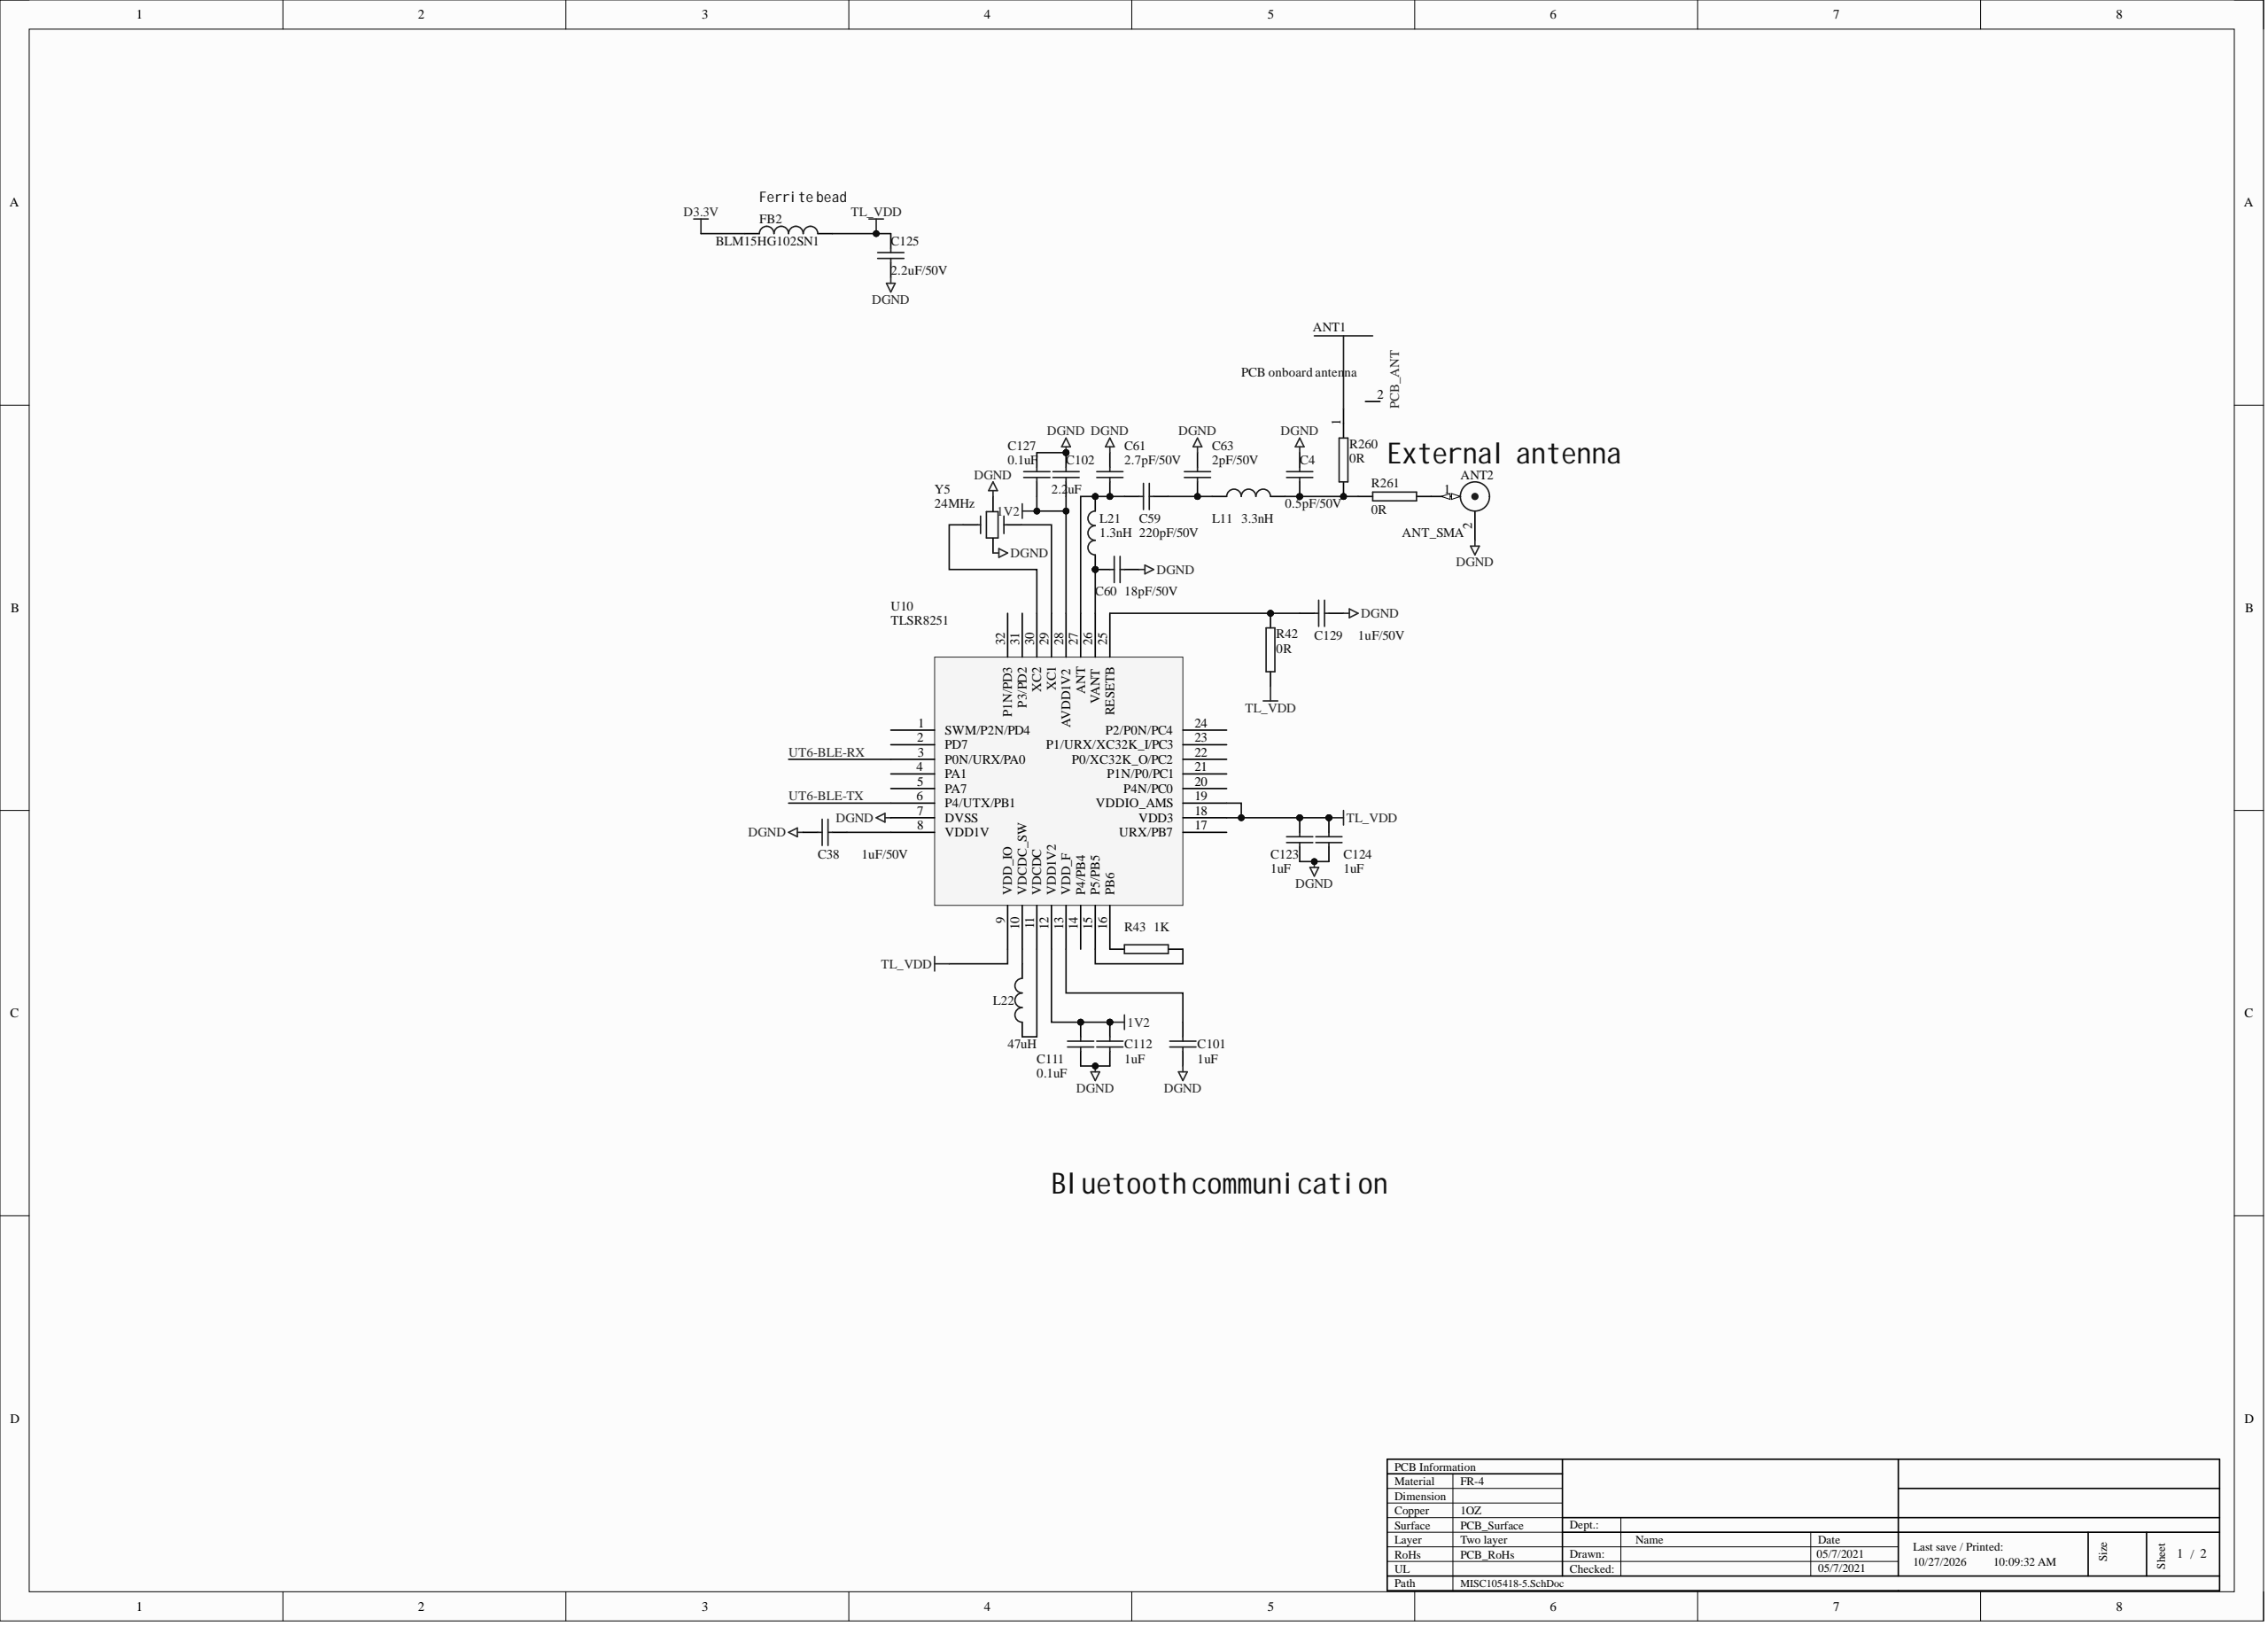Circuit board | Altium Designer | 455 parts | 280 nets | one sheet of the schematic
Parts on this sheet (reference | value | footprint):
ANT1 | PCB onboard antenna | ATN
ANT2 | ANT_SMA | ATN-1
C4 | 0.5pF/50V | C0402-T
C38 | 1uF/50V | C0402-T
C59 | 220pF/50V | C0402-T
C60 | 18pF/50V | C0402-T
C61 | 2.7pF/50V | C0402-T
C63 | 2pF/50V | C0402-T
C101 | 1uF | C0402-T
C102 | 2.2uF | C0402-T
C111 | 0.1uF | C0402-T
C112 | 1uF | C0402-T
C123 | 1uF | C0402-T
C124 | 1uF | C0402-T
C125 | 2.2uF/50V | C0603-T
C127 | 0.1uF | C0402-T
C129 | 1uF/50V | C0402-T
FB2 | BLM15HG102SN1 | R0603-T
L11 | 3.3nH | R0402-T
L21 | 1.3nH | R0402-T
L22 | 47uH | R0805-T
R42 | 0R | R0402-T
R43 | 1K | R0402-T
R260 | 0R | R0402-T
R261 | 0R | R0402-T
U10 | TLSR8251 | QFN32 5X5MM
Y5 | 24MHz | 23047-00020-11 32M SMD晶振
Nets of these parts (net: part-pin ...):
UT6-BLE-TX: U10-6
UT6-BLE-RX: U10-3
TL_VDD: C123-1 C124-1 C125-1 FB2-2 R42-1 U10-9 U10-18 U10-19
NetU10_30: U10-30 Y5-3
NetU10_29: U10-29 Y5-1
NetR43_2: R43-2 U10-16
NetR43_1: R43-1 U10-15
NetL22_2: L22-2 U10-11
NetL22_1: L22-1 U10-10
NetC129_1: C129-1 R42-2 U10-25
NetC101_1: C101-1 U10-13
NetC60_2: C60-2 L21-1 U10-26
NetC59_2: C59-2 C61-2 L21-2 U10-27
NetC59_1: C59-1 C63-2 L11-2
NetC38_2: C38-2 U10-8
NetC4_1: C4-1 L11-1 R260-2 R261-1
NetANT2_1: ANT2-1 R261-2
NetANT1_1: ANT1-1 R260-1
D3.3V: FB2-1
-: ANT2-2 C4-2 C38-1 C60-1 C61-1 C63-1 C101-2 C102-1 C111-2 C112-2 C123-2 C124-2 C125-2 C127-1 C129-2 U10-7 Y5-2 Y5-4
1V2: C102-2 C111-1 C112-1 C127-2 U10-12 U10-28